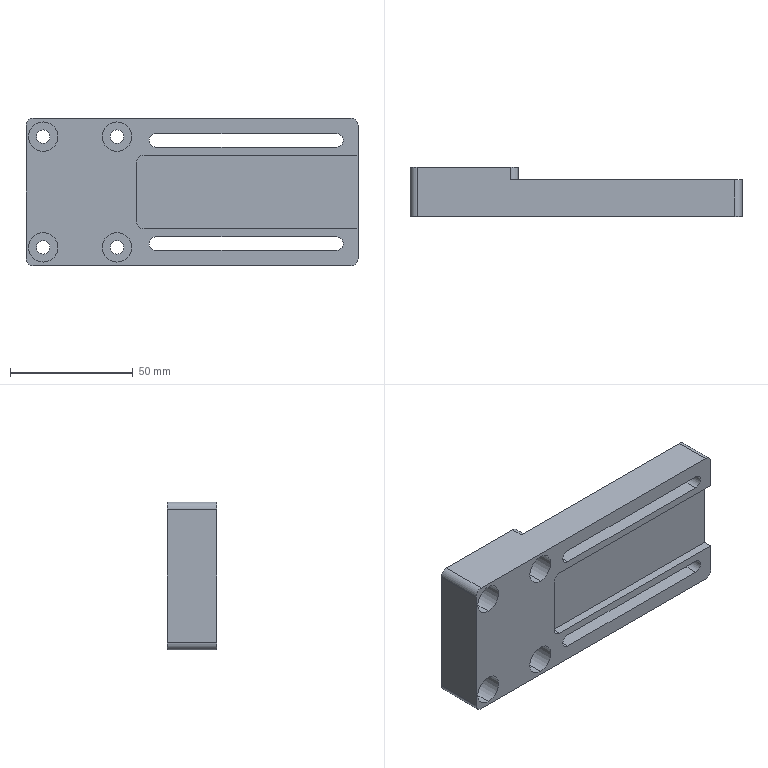Part | NX | features BREP 1 | 1 solid | 58 faces | box 135 x 20 x 60 mm | volume 98855 mm3 | cylinder 32 | plane 26 | commonest cylinder face diameters 5.5 x12 12 x12 6 x8